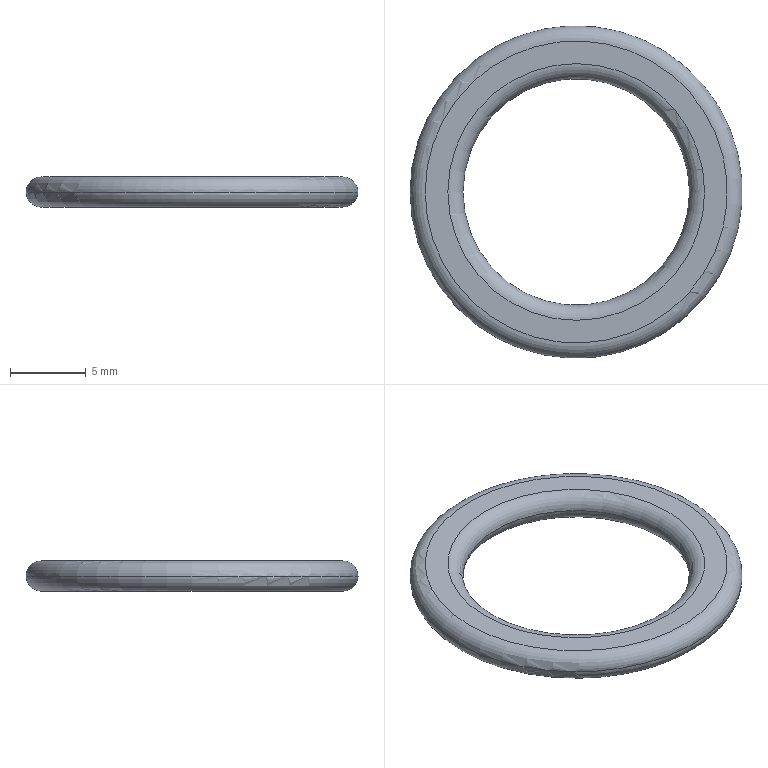Part | NX | features 模具.stp<1>[63] 2 | 1 solid | 6 faces | box 22 x 22 x 2 mm | volume 356.946 mm3 | torus 4 | plane 2
STEP:
#1=CARTESIAN_POINT('',(150.,25.,70.));
#2=VERTEX_POINT('',#1);
#3=CARTESIAN_POINT('',(160.,25.,70.));
#4=DIRECTION('',(0.,0.,-1.));
#5=DIRECTION('',(-1.,0.,0.));
#6=AXIS2_PLACEMENT_3D('',#3,#4,#5);
#7=CIRCLE('',#6,10.);
#8=EDGE_CURVE('',#2,#2,#7,.T.);
#9=ORIENTED_EDGE('',*,*,#8,.F.);
#10=EDGE_LOOP('',(#9));
#11=FACE_BOUND('',#10,.T.);
#12=CARTESIAN_POINT('',(149.,25.,71.));
#13=VERTEX_POINT('',#12);
#14=CARTESIAN_POINT('',(160.,25.,71.));
#15=DIRECTION('',(0.,0.,-1.));
#16=DIRECTION('',(-1.,0.,0.));
#17=AXIS2_PLACEMENT_3D('',#14,#15,#16);
#18=CIRCLE('',#17,11.);
#19=EDGE_CURVE('',#13,#13,#18,.T.);
#20=ORIENTED_EDGE('',*,*,#19,.T.);
#21=EDGE_LOOP('',(#20));
#22=FACE_BOUND('',#21,.T.);
#23=CARTESIAN_POINT('',(160.,25.,71.));
#24=DIRECTION('',(0.,0.,-1.));
#25=DIRECTION('',(-1.,0.,0.));
#26=AXIS2_PLACEMENT_3D('',#23,#24,#25);
#27=TOROIDAL_SURFACE('',#26,10.,1.);
#28=ADVANCED_FACE('',(#11,#22),#27,.T.);
#29=ORIENTED_EDGE('',*,*,#19,.F.);
#30=EDGE_LOOP('',(#29));
#31=FACE_BOUND('',#30,.T.);
#32=CARTESIAN_POINT('',(150.,25.,72.));
#33=VERTEX_POINT('',#32);
#34=CARTESIAN_POINT('',(160.,25.,72.));
#35=DIRECTION('',(0.,0.,1.));
#36=DIRECTION('',(-1.,0.,0.));
#37=AXIS2_PLACEMENT_3D('',#34,#35,#36);
#38=CIRCLE('',#37,10.);
#39=EDGE_CURVE('',#33,#33,#38,.T.);
#40=ORIENTED_EDGE('',*,*,#39,.F.);
#41=EDGE_LOOP('',(#40));
#42=FACE_BOUND('',#41,.T.);
#43=CARTESIAN_POINT('',(160.,25.,71.));
#44=DIRECTION('',(0.,0.,-1.));
#45=DIRECTION('',(-1.,0.,0.));
#46=AXIS2_PLACEMENT_3D('',#43,#44,#45);
#47=TOROIDAL_SURFACE('',#46,10.,1.);
#48=ADVANCED_FACE('',(#31,#42),#47,.T.);
#49=CARTESIAN_POINT('',(152.5,25.,71.));
#50=VERTEX_POINT('',#49);
#51=CARTESIAN_POINT('',(160.,25.,71.));
#52=DIRECTION('',(0.,0.,1.));
#53=DIRECTION('',(-1.,0.,0.));
#54=AXIS2_PLACEMENT_3D('',#51,#52,#53);
#55=CIRCLE('',#54,7.5);
#56=EDGE_CURVE('',#50,#50,#55,.T.);
#57=ORIENTED_EDGE('',*,*,#56,.T.);
#58=EDGE_LOOP('',(#57));
#59=FACE_BOUND('',#58,.T.);
#60=CARTESIAN_POINT('',(151.5,25.,70.));
#61=VERTEX_POINT('',#60);
#62=CARTESIAN_POINT('',(160.,25.,70.));
#63=DIRECTION('',(0.,0.,1.));
#64=DIRECTION('',(-1.,0.,0.));
#65=AXIS2_PLACEMENT_3D('',#62,#63,#64);
#66=CIRCLE('',#65,8.5);
#67=EDGE_CURVE('',#61,#61,#66,.T.);
#68=ORIENTED_EDGE('',*,*,#67,.F.);
#69=EDGE_LOOP('',(#68));
#70=FACE_BOUND('',#69,.T.);
#71=CARTESIAN_POINT('',(160.,25.,71.));
#72=DIRECTION('',(0.,0.,-1.));
#73=DIRECTION('',(-1.,0.,0.));
#74=AXIS2_PLACEMENT_3D('',#71,#72,#73);
#75=TOROIDAL_SURFACE('',#74,8.5,1.);
#76=ADVANCED_FACE('',(#59,#70),#75,.T.);
#77=ORIENTED_EDGE('',*,*,#56,.F.);
#78=EDGE_LOOP('',(#77));
#79=FACE_BOUND('',#78,.T.);
#80=CARTESIAN_POINT('',(151.5,25.,72.));
#81=VERTEX_POINT('',#80);
#82=CARTESIAN_POINT('',(160.,25.,72.));
#83=DIRECTION('',(0.,0.,-1.));
#84=DIRECTION('',(-1.,0.,0.));
#85=AXIS2_PLACEMENT_3D('',#82,#83,#84);
#86=CIRCLE('',#85,8.5);
#87=EDGE_CURVE('',#81,#81,#86,.T.);
#88=ORIENTED_EDGE('',*,*,#87,.F.);
#89=EDGE_LOOP('',(#88));
#90=FACE_BOUND('',#89,.T.);
#91=CARTESIAN_POINT('',(160.,25.,71.));
#92=DIRECTION('',(0.,0.,-1.));
#93=DIRECTION('',(-1.,0.,0.));
#94=AXIS2_PLACEMENT_3D('',#91,#92,#93);
#95=TOROIDAL_SURFACE('',#94,8.5,1.);
#96=ADVANCED_FACE('',(#79,#90),#95,.T.);
#97=ORIENTED_EDGE('',*,*,#39,.T.);
#98=EDGE_LOOP('',(#97));
#99=FACE_BOUND('',#98,.T.);
#100=ORIENTED_EDGE('',*,*,#87,.T.);
#101=EDGE_LOOP('',(#100));
#102=FACE_BOUND('',#101,.T.);
#103=CARTESIAN_POINT('',(160.,25.,72.));
#104=DIRECTION('',(0.,0.,-1.));
#105=DIRECTION('',(0.,-1.,0.));
#106=AXIS2_PLACEMENT_3D('',#103,#104,#105);
#107=PLANE('',#106);
#108=ADVANCED_FACE('',(#99,#102),#107,.F.);
#109=ORIENTED_EDGE('',*,*,#8,.T.);
#110=EDGE_LOOP('',(#109));
#111=FACE_BOUND('',#110,.T.);
#112=ORIENTED_EDGE('',*,*,#67,.T.);
#113=EDGE_LOOP('',(#112));
#114=FACE_BOUND('',#113,.T.);
#115=CARTESIAN_POINT('',(160.,25.,70.));
#116=DIRECTION('',(0.,0.,-1.));
#117=DIRECTION('',(0.,-1.,0.));
#118=AXIS2_PLACEMENT_3D('',#115,#116,#117);
#119=PLANE('',#118);
#120=ADVANCED_FACE('',(#111,#114),#119,.T.);
#121=CLOSED_SHELL('',(#28,#48,#76,#96,#108,#120));
#122=MANIFOLD_SOLID_BREP('',#121);
#123=(LENGTH_UNIT()NAMED_UNIT(*)SI_UNIT(.MILLI.,.METRE.));
#124=UNCERTAINTY_MEASURE_WITH_UNIT(LENGTH_MEASURE(0.00001),#123,'','');
#125=(NAMED_UNIT(*)PLANE_ANGLE_UNIT()SI_UNIT($,.RADIAN.));
#126=(NAMED_UNIT(*)SI_UNIT($,.STERADIAN.)SOLID_ANGLE_UNIT());
#127=(GEOMETRIC_REPRESENTATION_CONTEXT(3)GLOBAL_UNCERTAINTY_ASSIGNED_CONTEXT((#124))GLOBAL_UNIT_ASSIGNED_CONTEXT((#123,#125,#126))REPRESENTATION_CONTEXT('',''));
#128=ADVANCED_BREP_SHAPE_REPRESENTATION('',(#122),#127);